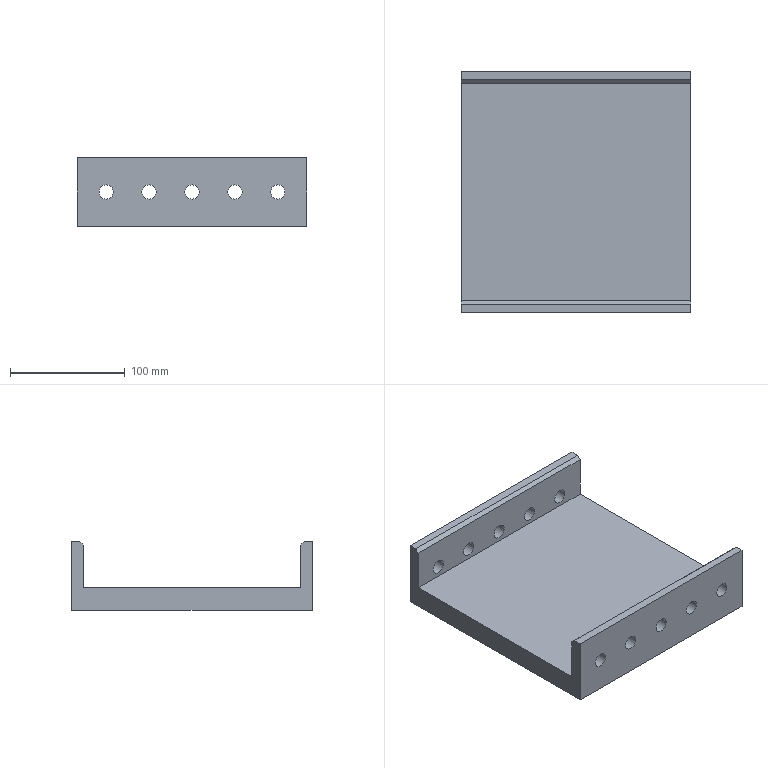Part | NX | features SIMPLE HOLE 15, DATUM_CSYS 7, SKETCH 6, EXTRACT_BODY 5, EXTRACT_DATUM_AXIS 5, EXTRACT_FACE 5, HOLE PACKAGE 5, Instance Feature 4, CHAMFER 2, Delete Body 2, EXTRUDE 2, Container 1, Geometry Instance 1, Pattern Feature 1, SUBTRACT 1 | 1 solid | 22 faces | box 200 x 210 x 60 mm | volume 985928 mm3 | plane 12 | cylinder 10 | commonest cylinder face diameters 12.5 x10
STEP:
#1=CARTESIAN_POINT('',(25.,200.,36.25));
#2=VERTEX_POINT('',#1);
#3=CARTESIAN_POINT('',(25.,200.,30.));
#4=DIRECTION('',(0.,1.,0.));
#5=DIRECTION('',(0.,0.,1.));
#6=AXIS2_PLACEMENT_3D('',#3,#4,#5);
#7=CIRCLE('',#6,6.25);
#8=EDGE_CURVE('',#2,#2,#7,.T.);
#9=ORIENTED_EDGE('',*,*,#8,.T.);
#10=EDGE_LOOP('',(#9));
#11=FACE_BOUND('',#10,.T.);
#12=CARTESIAN_POINT('',(62.5,200.,36.25));
#13=VERTEX_POINT('',#12);
#14=CARTESIAN_POINT('',(62.5,200.,30.));
#15=DIRECTION('',(0.,1.,0.));
#16=DIRECTION('',(0.,0.,1.));
#17=AXIS2_PLACEMENT_3D('',#14,#15,#16);
#18=CIRCLE('',#17,6.25);
#19=EDGE_CURVE('',#13,#13,#18,.T.);
#20=ORIENTED_EDGE('',*,*,#19,.T.);
#21=EDGE_LOOP('',(#20));
#22=FACE_BOUND('',#21,.T.);
#23=CARTESIAN_POINT('',(100.,200.,36.25));
#24=VERTEX_POINT('',#23);
#25=CARTESIAN_POINT('',(100.,200.,30.));
#26=DIRECTION('',(0.,1.,0.));
#27=DIRECTION('',(0.,0.,1.));
#28=AXIS2_PLACEMENT_3D('',#25,#26,#27);
#29=CIRCLE('',#28,6.25);
#30=EDGE_CURVE('',#24,#24,#29,.T.);
#31=ORIENTED_EDGE('',*,*,#30,.T.);
#32=EDGE_LOOP('',(#31));
#33=FACE_BOUND('',#32,.T.);
#34=CARTESIAN_POINT('',(137.5,200.,36.25));
#35=VERTEX_POINT('',#34);
#36=CARTESIAN_POINT('',(137.5,200.,30.));
#37=DIRECTION('',(0.,1.,0.));
#38=DIRECTION('',(0.,0.,1.));
#39=AXIS2_PLACEMENT_3D('',#36,#37,#38);
#40=CIRCLE('',#39,6.25);
#41=EDGE_CURVE('',#35,#35,#40,.T.);
#42=ORIENTED_EDGE('',*,*,#41,.T.);
#43=EDGE_LOOP('',(#42));
#44=FACE_BOUND('',#43,.T.);
#45=CARTESIAN_POINT('',(175.,200.,36.25));
#46=VERTEX_POINT('',#45);
#47=CARTESIAN_POINT('',(175.,200.,30.));
#48=DIRECTION('',(0.,1.,0.));
#49=DIRECTION('',(0.,0.,1.));
#50=AXIS2_PLACEMENT_3D('',#47,#48,#49);
#51=CIRCLE('',#50,6.25);
#52=EDGE_CURVE('',#46,#46,#51,.T.);
#53=ORIENTED_EDGE('',*,*,#52,.T.);
#54=EDGE_LOOP('',(#53));
#55=FACE_BOUND('',#54,.T.);
#56=CARTESIAN_POINT('',(200.,200.,57.));
#57=VERTEX_POINT('',#56);
#58=CARTESIAN_POINT('',(200.,200.,20.));
#59=VERTEX_POINT('',#58);
#60=CARTESIAN_POINT('',(200.,200.,60.));
#61=DIRECTION('',(0.,0.,-1.));
#62=VECTOR('',#61,1000.);
#63=LINE('',#60,#62);
#64=EDGE_CURVE('',#57,#59,#63,.T.);
#65=ORIENTED_EDGE('',*,*,#64,.F.);
#66=CARTESIAN_POINT('',(0.,200.,57.));
#67=VERTEX_POINT('',#66);
#68=CARTESIAN_POINT('',(200.,200.,57.));
#69=DIRECTION('',(-1.,0.,0.));
#70=VECTOR('',#69,1000.);
#71=LINE('',#68,#70);
#72=EDGE_CURVE('',#57,#67,#71,.T.);
#73=ORIENTED_EDGE('',*,*,#72,.T.);
#74=CARTESIAN_POINT('',(0.,200.,20.));
#75=VERTEX_POINT('',#74);
#76=CARTESIAN_POINT('',(0.,200.,60.));
#77=DIRECTION('',(0.,0.,-1.));
#78=VECTOR('',#77,1000.);
#79=LINE('',#76,#78);
#80=EDGE_CURVE('',#67,#75,#79,.T.);
#81=ORIENTED_EDGE('',*,*,#80,.T.);
#82=CARTESIAN_POINT('',(200.,200.,20.));
#83=DIRECTION('',(-1.,0.,0.));
#84=VECTOR('',#83,1000.);
#85=LINE('',#82,#84);
#86=EDGE_CURVE('',#59,#75,#85,.T.);
#87=ORIENTED_EDGE('',*,*,#86,.F.);
#88=EDGE_LOOP('',(#65,#73,#81,#87));
#89=FACE_BOUND('',#88,.T.);
#90=CARTESIAN_POINT('',(200.,200.,60.));
#91=DIRECTION('',(0.,1.,0.));
#92=DIRECTION('',(0.,0.,1.));
#93=AXIS2_PLACEMENT_3D('',#90,#91,#92);
#94=PLANE('',#93);
#95=ADVANCED_FACE('',(#11,#22,#33,#44,#55,#89),#94,.F.);
#96=CARTESIAN_POINT('',(25.,10.,36.25));
#97=VERTEX_POINT('',#96);
#98=CARTESIAN_POINT('',(25.,10.,30.));
#99=DIRECTION('',(0.,1.,0.));
#100=DIRECTION('',(0.,0.,1.));
#101=AXIS2_PLACEMENT_3D('',#98,#99,#100);
#102=CIRCLE('',#101,6.25);
#103=EDGE_CURVE('',#97,#97,#102,.F.);
#104=ORIENTED_EDGE('',*,*,#103,.T.);
#105=EDGE_LOOP('',(#104));
#106=FACE_BOUND('',#105,.T.);
#107=CARTESIAN_POINT('',(62.5,10.,36.25));
#108=VERTEX_POINT('',#107);
#109=CARTESIAN_POINT('',(62.5,10.,30.));
#110=DIRECTION('',(0.,1.,0.));
#111=DIRECTION('',(0.,0.,1.));
#112=AXIS2_PLACEMENT_3D('',#109,#110,#111);
#113=CIRCLE('',#112,6.25);
#114=EDGE_CURVE('',#108,#108,#113,.F.);
#115=ORIENTED_EDGE('',*,*,#114,.T.);
#116=EDGE_LOOP('',(#115));
#117=FACE_BOUND('',#116,.T.);
#118=CARTESIAN_POINT('',(100.,10.,36.25));
#119=VERTEX_POINT('',#118);
#120=CARTESIAN_POINT('',(100.,10.,30.));
#121=DIRECTION('',(0.,1.,0.));
#122=DIRECTION('',(0.,0.,1.));
#123=AXIS2_PLACEMENT_3D('',#120,#121,#122);
#124=CIRCLE('',#123,6.25);
#125=EDGE_CURVE('',#119,#119,#124,.F.);
#126=ORIENTED_EDGE('',*,*,#125,.T.);
#127=EDGE_LOOP('',(#126));
#128=FACE_BOUND('',#127,.T.);
#129=CARTESIAN_POINT('',(175.,10.,36.25));
#130=VERTEX_POINT('',#129);
#131=CARTESIAN_POINT('',(175.,10.,30.));
#132=DIRECTION('',(0.,1.,0.));
#133=DIRECTION('',(0.,0.,1.));
#134=AXIS2_PLACEMENT_3D('',#131,#132,#133);
#135=CIRCLE('',#134,6.25);
#136=EDGE_CURVE('',#130,#130,#135,.F.);
#137=ORIENTED_EDGE('',*,*,#136,.T.);
#138=EDGE_LOOP('',(#137));
#139=FACE_BOUND('',#138,.T.);
#140=CARTESIAN_POINT('',(137.5,10.,36.25));
#141=VERTEX_POINT('',#140);
#142=CARTESIAN_POINT('',(137.5,10.,30.));
#143=DIRECTION('',(0.,1.,0.));
#144=DIRECTION('',(0.,0.,1.));
#145=AXIS2_PLACEMENT_3D('',#142,#143,#144);
#146=CIRCLE('',#145,6.25);
#147=EDGE_CURVE('',#141,#141,#146,.F.);
#148=ORIENTED_EDGE('',*,*,#147,.T.);
#149=EDGE_LOOP('',(#148));
#150=FACE_BOUND('',#149,.T.);
#151=CARTESIAN_POINT('',(0.,10.,20.));
#152=VERTEX_POINT('',#151);
#153=CARTESIAN_POINT('',(0.,10.,57.));
#154=VERTEX_POINT('',#153);
#155=CARTESIAN_POINT('',(0.,10.,10.));
#156=DIRECTION('',(0.,0.,1.));
#157=VECTOR('',#156,1000.);
#158=LINE('',#155,#157);
#159=EDGE_CURVE('',#152,#154,#158,.T.);
#160=ORIENTED_EDGE('',*,*,#159,.T.);
#161=CARTESIAN_POINT('',(200.,10.,57.));
#162=VERTEX_POINT('',#161);
#163=CARTESIAN_POINT('',(200.,10.,57.));
#164=DIRECTION('',(1.,0.,0.));
#165=VECTOR('',#164,1000.);
#166=LINE('',#163,#165);
#167=EDGE_CURVE('',#154,#162,#166,.T.);
#168=ORIENTED_EDGE('',*,*,#167,.T.);
#169=CARTESIAN_POINT('',(200.,10.,20.));
#170=VERTEX_POINT('',#169);
#171=CARTESIAN_POINT('',(200.,10.,10.));
#172=DIRECTION('',(0.,0.,1.));
#173=VECTOR('',#172,1000.);
#174=LINE('',#171,#173);
#175=EDGE_CURVE('',#170,#162,#174,.T.);
#176=ORIENTED_EDGE('',*,*,#175,.F.);
#177=CARTESIAN_POINT('',(0.,10.,20.));
#178=DIRECTION('',(1.,0.,0.));
#179=VECTOR('',#178,1000.);
#180=LINE('',#177,#179);
#181=EDGE_CURVE('',#152,#170,#180,.T.);
#182=ORIENTED_EDGE('',*,*,#181,.F.);
#183=EDGE_LOOP('',(#160,#168,#176,#182));
#184=FACE_BOUND('',#183,.T.);
#185=CARTESIAN_POINT('',(200.,10.,10.));
#186=DIRECTION('',(0.,-1.,0.));
#187=DIRECTION('',(0.,0.,-1.));
#188=AXIS2_PLACEMENT_3D('',#185,#186,#187);
#189=PLANE('',#188);
#190=ADVANCED_FACE('',(#106,#117,#128,#139,#150,#184),#189,.F.);
#191=CARTESIAN_POINT('',(137.5,0.,23.75));
#192=VERTEX_POINT('',#191);
#193=CARTESIAN_POINT('',(137.5,0.,30.));
#194=DIRECTION('',(0.,-1.,0.));
#195=DIRECTION('',(0.,0.,-1.));
#196=AXIS2_PLACEMENT_3D('',#193,#194,#195);
#197=CIRCLE('',#196,6.25);
#198=EDGE_CURVE('',#192,#192,#197,.T.);
#199=ORIENTED_EDGE('',*,*,#198,.F.);
#200=EDGE_LOOP('',(#199));
#201=FACE_BOUND('',#200,.T.);
#202=CARTESIAN_POINT('',(175.,0.,23.75));
#203=VERTEX_POINT('',#202);
#204=CARTESIAN_POINT('',(175.,0.,30.));
#205=DIRECTION('',(0.,-1.,0.));
#206=DIRECTION('',(0.,0.,-1.));
#207=AXIS2_PLACEMENT_3D('',#204,#205,#206);
#208=CIRCLE('',#207,6.25);
#209=EDGE_CURVE('',#203,#203,#208,.T.);
#210=ORIENTED_EDGE('',*,*,#209,.F.);
#211=EDGE_LOOP('',(#210));
#212=FACE_BOUND('',#211,.T.);
#213=CARTESIAN_POINT('',(100.,0.,23.75));
#214=VERTEX_POINT('',#213);
#215=CARTESIAN_POINT('',(100.,0.,30.));
#216=DIRECTION('',(0.,-1.,0.));
#217=DIRECTION('',(0.,0.,-1.));
#218=AXIS2_PLACEMENT_3D('',#215,#216,#217);
#219=CIRCLE('',#218,6.25);
#220=EDGE_CURVE('',#214,#214,#219,.T.);
#221=ORIENTED_EDGE('',*,*,#220,.F.);
#222=EDGE_LOOP('',(#221));
#223=FACE_BOUND('',#222,.T.);
#224=CARTESIAN_POINT('',(62.5,0.,23.75));
#225=VERTEX_POINT('',#224);
#226=CARTESIAN_POINT('',(62.5,0.,30.));
#227=DIRECTION('',(0.,-1.,0.));
#228=DIRECTION('',(0.,0.,-1.));
#229=AXIS2_PLACEMENT_3D('',#226,#227,#228);
#230=CIRCLE('',#229,6.25);
#231=EDGE_CURVE('',#225,#225,#230,.T.);
#232=ORIENTED_EDGE('',*,*,#231,.F.);
#233=EDGE_LOOP('',(#232));
#234=FACE_BOUND('',#233,.T.);
#235=CARTESIAN_POINT('',(25.,0.,23.75));
#236=VERTEX_POINT('',#235);
#237=CARTESIAN_POINT('',(25.,0.,30.));
#238=DIRECTION('',(0.,-1.,0.));
#239=DIRECTION('',(0.,0.,-1.));
#240=AXIS2_PLACEMENT_3D('',#237,#238,#239);
#241=CIRCLE('',#240,6.25);
#242=EDGE_CURVE('',#236,#236,#241,.T.);
#243=ORIENTED_EDGE('',*,*,#242,.F.);
#244=EDGE_LOOP('',(#243));
#245=FACE_BOUND('',#244,.T.);
#246=CARTESIAN_POINT('',(0.,0.,60.));
#247=VERTEX_POINT('',#246);
#248=CARTESIAN_POINT('',(0.,0.,0.));
#249=VERTEX_POINT('',#248);
#250=CARTESIAN_POINT('',(0.,0.,60.));
#251=DIRECTION('',(0.,0.,-1.));
#252=VECTOR('',#251,1000.);
#253=LINE('',#250,#252);
#254=EDGE_CURVE('',#247,#249,#253,.T.);
#255=ORIENTED_EDGE('',*,*,#254,.T.);
#256=CARTESIAN_POINT('',(200.,0.,0.));
#257=VERTEX_POINT('',#256);
#258=CARTESIAN_POINT('',(200.,0.,0.));
#259=DIRECTION('',(-1.,0.,0.));
#260=VECTOR('',#259,1000.);
#261=LINE('',#258,#260);
#262=EDGE_CURVE('',#257,#249,#261,.T.);
#263=ORIENTED_EDGE('',*,*,#262,.F.);
#264=CARTESIAN_POINT('',(200.,0.,60.));
#265=VERTEX_POINT('',#264);
#266=CARTESIAN_POINT('',(200.,0.,60.));
#267=DIRECTION('',(0.,0.,-1.));
#268=VECTOR('',#267,1000.);
#269=LINE('',#266,#268);
#270=EDGE_CURVE('',#265,#257,#269,.T.);
#271=ORIENTED_EDGE('',*,*,#270,.F.);
#272=CARTESIAN_POINT('',(200.,0.,60.));
#273=DIRECTION('',(-1.,0.,0.));
#274=VECTOR('',#273,1000.);
#275=LINE('',#272,#274);
#276=EDGE_CURVE('',#265,#247,#275,.T.);
#277=ORIENTED_EDGE('',*,*,#276,.T.);
#278=EDGE_LOOP('',(#255,#263,#271,#277));
#279=FACE_BOUND('',#278,.T.);
#280=CARTESIAN_POINT('',(200.,0.,60.));
#281=DIRECTION('',(0.,1.,0.));
#282=DIRECTION('',(0.,0.,1.));
#283=AXIS2_PLACEMENT_3D('',#280,#281,#282);
#284=PLANE('',#283);
#285=ADVANCED_FACE('',(#201,#212,#223,#234,#245,#279),#284,.F.);
#286=CARTESIAN_POINT('',(0.,210.,0.));
#287=VERTEX_POINT('',#286);
#288=CARTESIAN_POINT('',(0.,0.,0.));
#289=DIRECTION('',(0.,1.,0.));
#290=VECTOR('',#289,1000.);
#291=LINE('',#288,#290);
#292=EDGE_CURVE('',#249,#287,#291,.T.);
#293=ORIENTED_EDGE('',*,*,#292,.T.);
#294=CARTESIAN_POINT('',(200.,210.,0.));
#295=VERTEX_POINT('',#294);
#296=CARTESIAN_POINT('',(200.,210.,0.));
#297=DIRECTION('',(-1.,0.,0.));
#298=VECTOR('',#297,1000.);
#299=LINE('',#296,#298);
#300=EDGE_CURVE('',#295,#287,#299,.T.);
#301=ORIENTED_EDGE('',*,*,#300,.F.);
#302=CARTESIAN_POINT('',(200.,0.,0.));
#303=DIRECTION('',(0.,1.,0.));
#304=VECTOR('',#303,1000.);
#305=LINE('',#302,#304);
#306=EDGE_CURVE('',#257,#295,#305,.T.);
#307=ORIENTED_EDGE('',*,*,#306,.F.);
#308=ORIENTED_EDGE('',*,*,#262,.T.);
#309=EDGE_LOOP('',(#293,#301,#307,#308));
#310=FACE_BOUND('',#309,.T.);
#311=CARTESIAN_POINT('',(200.,0.,0.));
#312=DIRECTION('',(0.,0.,1.));
#313=DIRECTION('',(0.,-1.,0.));
#314=AXIS2_PLACEMENT_3D('',#311,#312,#313);
#315=PLANE('',#314);
#316=ADVANCED_FACE('',(#310),#315,.F.);
#317=CARTESIAN_POINT('',(175.,210.,23.75));
#318=VERTEX_POINT('',#317);
#319=CARTESIAN_POINT('',(175.,210.,30.));
#320=DIRECTION('',(0.,-1.,0.));
#321=DIRECTION('',(0.,0.,-1.));
#322=AXIS2_PLACEMENT_3D('',#319,#320,#321);
#323=CIRCLE('',#322,6.25);
#324=EDGE_CURVE('',#318,#318,#323,.F.);
#325=ORIENTED_EDGE('',*,*,#324,.F.);
#326=EDGE_LOOP('',(#325));
#327=FACE_BOUND('',#326,.T.);
#328=CARTESIAN_POINT('',(137.5,210.,23.75));
#329=VERTEX_POINT('',#328);
#330=CARTESIAN_POINT('',(137.5,210.,30.));
#331=DIRECTION('',(0.,-1.,0.));
#332=DIRECTION('',(0.,0.,-1.));
#333=AXIS2_PLACEMENT_3D('',#330,#331,#332);
#334=CIRCLE('',#333,6.25);
#335=EDGE_CURVE('',#329,#329,#334,.F.);
#336=ORIENTED_EDGE('',*,*,#335,.F.);
#337=EDGE_LOOP('',(#336));
#338=FACE_BOUND('',#337,.T.);
#339=CARTESIAN_POINT('',(100.,210.,23.75));
#340=VERTEX_POINT('',#339);
#341=CARTESIAN_POINT('',(100.,210.,30.));
#342=DIRECTION('',(0.,-1.,0.));
#343=DIRECTION('',(0.,0.,-1.));
#344=AXIS2_PLACEMENT_3D('',#341,#342,#343);
#345=CIRCLE('',#344,6.25);
#346=EDGE_CURVE('',#340,#340,#345,.F.);
#347=ORIENTED_EDGE('',*,*,#346,.F.);
#348=EDGE_LOOP('',(#347));
#349=FACE_BOUND('',#348,.T.);
#350=CARTESIAN_POINT('',(62.5,210.,23.75));
#351=VERTEX_POINT('',#350);
#352=CARTESIAN_POINT('',(62.5,210.,30.));
#353=DIRECTION('',(0.,-1.,0.));
#354=DIRECTION('',(0.,0.,-1.));
#355=AXIS2_PLACEMENT_3D('',#352,#353,#354);
#356=CIRCLE('',#355,6.25);
#357=EDGE_CURVE('',#351,#351,#356,.F.);
#358=ORIENTED_EDGE('',*,*,#357,.F.);
#359=EDGE_LOOP('',(#358));
#360=FACE_BOUND('',#359,.T.);
#361=CARTESIAN_POINT('',(25.,210.,23.75));
#362=VERTEX_POINT('',#361);
#363=CARTESIAN_POINT('',(25.,210.,30.));
#364=DIRECTION('',(0.,-1.,0.));
#365=DIRECTION('',(0.,0.,-1.));
#366=AXIS2_PLACEMENT_3D('',#363,#364,#365);
#367=CIRCLE('',#366,6.25);
#368=EDGE_CURVE('',#362,#362,#367,.T.);
#369=ORIENTED_EDGE('',*,*,#368,.T.);
#370=EDGE_LOOP('',(#369));
#371=FACE_BOUND('',#370,.T.);
#372=CARTESIAN_POINT('',(0.,210.,60.));
#373=VERTEX_POINT('',#372);
#374=CARTESIAN_POINT('',(0.,210.,0.));
#375=DIRECTION('',(0.,0.,1.));
#376=VECTOR('',#375,1000.);
#377=LINE('',#374,#376);
#378=EDGE_CURVE('',#287,#373,#377,.T.);
#379=ORIENTED_EDGE('',*,*,#378,.T.);
#380=CARTESIAN_POINT('',(200.,210.,60.));
#381=VERTEX_POINT('',#380);
#382=CARTESIAN_POINT('',(200.,210.,60.));
#383=DIRECTION('',(-1.,0.,0.));
#384=VECTOR('',#383,1000.);
#385=LINE('',#382,#384);
#386=EDGE_CURVE('',#381,#373,#385,.T.);
#387=ORIENTED_EDGE('',*,*,#386,.F.);
#388=CARTESIAN_POINT('',(200.,210.,0.));
#389=DIRECTION('',(0.,0.,1.));
#390=VECTOR('',#389,1000.);
#391=LINE('',#388,#390);
#392=EDGE_CURVE('',#295,#381,#391,.T.);
#393=ORIENTED_EDGE('',*,*,#392,.F.);
#394=ORIENTED_EDGE('',*,*,#300,.T.);
#395=EDGE_LOOP('',(#379,#387,#393,#394));
#396=FACE_BOUND('',#395,.T.);
#397=CARTESIAN_POINT('',(200.,210.,0.));
#398=DIRECTION('',(0.,-1.,0.));
#399=DIRECTION('',(0.,0.,-1.));
#400=AXIS2_PLACEMENT_3D('',#397,#398,#399);
#401=PLANE('',#400);
#402=ADVANCED_FACE('',(#327,#338,#349,#360,#371,#396),#401,.F.);
#403=CARTESIAN_POINT('',(0.,203.,60.));
#404=VERTEX_POINT('',#403);
#405=CARTESIAN_POINT('',(0.,210.,60.));
#406=DIRECTION('',(0.,-1.,0.));
#407=VECTOR('',#406,1000.);
#408=LINE('',#405,#407);
#409=EDGE_CURVE('',#373,#404,#408,.T.);
#410=ORIENTED_EDGE('',*,*,#409,.T.);
#411=CARTESIAN_POINT('',(200.,203.,60.));
#412=VERTEX_POINT('',#411);
#413=CARTESIAN_POINT('',(200.,203.,60.));
#414=DIRECTION('',(1.,0.,0.));
#415=VECTOR('',#414,1000.);
#416=LINE('',#413,#415);
#417=EDGE_CURVE('',#404,#412,#416,.T.);
#418=ORIENTED_EDGE('',*,*,#417,.T.);
#419=CARTESIAN_POINT('',(200.,210.,60.));
#420=DIRECTION('',(0.,-1.,0.));
#421=VECTOR('',#420,1000.);
#422=LINE('',#419,#421);
#423=EDGE_CURVE('',#381,#412,#422,.T.);
#424=ORIENTED_EDGE('',*,*,#423,.F.);
#425=ORIENTED_EDGE('',*,*,#386,.T.);
#426=EDGE_LOOP('',(#410,#418,#424,#425));
#427=FACE_BOUND('',#426,.T.);
#428=CARTESIAN_POINT('',(200.,210.,60.));
#429=DIRECTION('',(0.,0.,-1.));
#430=DIRECTION('',(-1.,0.,0.));
#431=AXIS2_PLACEMENT_3D('',#428,#429,#430);
#432=PLANE('',#431);
#433=ADVANCED_FACE('',(#427),#432,.F.);
#434=CARTESIAN_POINT('',(200.,7.,60.));
#435=VERTEX_POINT('',#434);
#436=CARTESIAN_POINT('',(200.,10.,60.));
#437=DIRECTION('',(0.,-1.,0.));
#438=VECTOR('',#437,1000.);
#439=LINE('',#436,#438);
#440=EDGE_CURVE('',#435,#265,#439,.T.);
#441=ORIENTED_EDGE('',*,*,#440,.F.);
#442=CARTESIAN_POINT('',(0.,7.,60.));
#443=VERTEX_POINT('',#442);
#444=CARTESIAN_POINT('',(200.,7.,60.));
#445=DIRECTION('',(-1.,0.,0.));
#446=VECTOR('',#445,1000.);
#447=LINE('',#444,#446);
#448=EDGE_CURVE('',#435,#443,#447,.T.);
#449=ORIENTED_EDGE('',*,*,#448,.T.);
#450=CARTESIAN_POINT('',(0.,10.,60.));
#451=DIRECTION('',(0.,-1.,0.));
#452=VECTOR('',#451,1000.);
#453=LINE('',#450,#452);
#454=EDGE_CURVE('',#443,#247,#453,.T.);
#455=ORIENTED_EDGE('',*,*,#454,.T.);
#456=ORIENTED_EDGE('',*,*,#276,.F.);
#457=EDGE_LOOP('',(#441,#449,#455,#456));
#458=FACE_BOUND('',#457,.T.);
#459=CARTESIAN_POINT('',(200.,10.,60.));
#460=DIRECTION('',(0.,0.,-1.));
#461=DIRECTION('',(-1.,0.,0.));
#462=AXIS2_PLACEMENT_3D('',#459,#460,#461);
#463=PLANE('',#462);
#464=ADVANCED_FACE('',(#458),#463,.F.);
#465=ORIENTED_EDGE('',*,*,#175,.T.);
#466=CARTESIAN_POINT('',(200.,33.5,33.5));
#467=DIRECTION('',(0.,0.7071,-0.7071));
#468=VECTOR('',#467,1000.);
#469=LINE('',#466,#468);
#470=EDGE_CURVE('',#162,#435,#469,.F.);
#471=ORIENTED_EDGE('',*,*,#470,.T.);
#472=ORIENTED_EDGE('',*,*,#440,.T.);
#473=ORIENTED_EDGE('',*,*,#270,.T.);
#474=ORIENTED_EDGE('',*,*,#306,.T.);
#475=ORIENTED_EDGE('',*,*,#392,.T.);
#476=ORIENTED_EDGE('',*,*,#423,.T.);
#477=CARTESIAN_POINT('',(200.,71.5,-71.5));
#478=DIRECTION('',(0.,0.7071,0.7071));
#479=VECTOR('',#478,1000.);
#480=LINE('',#477,#479);
#481=EDGE_CURVE('',#412,#57,#480,.F.);
#482=ORIENTED_EDGE('',*,*,#481,.T.);
#483=ORIENTED_EDGE('',*,*,#64,.T.);
#484=CARTESIAN_POINT('',(200.,10.,20.));
#485=DIRECTION('',(0.,1.,0.));
#486=VECTOR('',#485,1000.);
#487=LINE('',#484,#486);
#488=EDGE_CURVE('',#170,#59,#487,.T.);
#489=ORIENTED_EDGE('',*,*,#488,.F.);
#490=EDGE_LOOP('',(#465,#471,#472,#473,#474,#475,#476,#482,#483,#489));
#491=FACE_BOUND('',#490,.T.);
#492=CARTESIAN_POINT('',(200.,0.,0.));
#493=DIRECTION('',(1.,0.,0.));
#494=DIRECTION('',(0.,0.,-1.));
#495=AXIS2_PLACEMENT_3D('',#492,#493,#494);
#496=PLANE('',#495);
#497=ADVANCED_FACE('',(#491),#496,.T.);
#498=ORIENTED_EDGE('',*,*,#454,.F.);
#499=CARTESIAN_POINT('',(0.,7.,60.));
#500=DIRECTION('',(0.,-0.7071,0.7071));
#501=VECTOR('',#500,1000.);
#502=LINE('',#499,#501);
#503=EDGE_CURVE('',#443,#154,#502,.F.);
#504=ORIENTED_EDGE('',*,*,#503,.T.);
#505=ORIENTED_EDGE('',*,*,#159,.F.);
#506=CARTESIAN_POINT('',(0.,200.,20.));
#507=DIRECTION('',(0.,-1.,0.));
#508=VECTOR('',#507,1000.);
#509=LINE('',#506,#508);
#510=EDGE_CURVE('',#75,#152,#509,.T.);
#511=ORIENTED_EDGE('',*,*,#510,.F.);
#512=ORIENTED_EDGE('',*,*,#80,.F.);
#513=CARTESIAN_POINT('',(0.,200.,57.));
#514=DIRECTION('',(0.,-0.7071,-0.7071));
#515=VECTOR('',#514,1000.);
#516=LINE('',#513,#515);
#517=EDGE_CURVE('',#67,#404,#516,.F.);
#518=ORIENTED_EDGE('',*,*,#517,.T.);
#519=ORIENTED_EDGE('',*,*,#409,.F.);
#520=ORIENTED_EDGE('',*,*,#378,.F.);
#521=ORIENTED_EDGE('',*,*,#292,.F.);
#522=ORIENTED_EDGE('',*,*,#254,.F.);
#523=EDGE_LOOP('',(#498,#504,#505,#511,#512,#518,#519,#520,#521,#522));
#524=FACE_BOUND('',#523,.T.);
#525=CARTESIAN_POINT('',(0.,0.,0.));
#526=DIRECTION('',(1.,0.,0.));
#527=DIRECTION('',(0.,0.,-1.));
#528=AXIS2_PLACEMENT_3D('',#525,#526,#527);
#529=PLANE('',#528);
#530=ADVANCED_FACE('',(#524),#529,.F.);
#531=ORIENTED_EDGE('',*,*,#368,.F.);
#532=EDGE_LOOP('',(#531));
#533=FACE_BOUND('',#532,.T.);
#534=ORIENTED_EDGE('',*,*,#8,.F.);
#535=EDGE_LOOP('',(#534));
#536=FACE_BOUND('',#535,.T.);
#537=CARTESIAN_POINT('',(25.,200.,30.));
#538=DIRECTION('',(0.,1.,0.));
#539=DIRECTION('',(0.,0.,1.));
#540=AXIS2_PLACEMENT_3D('',#537,#538,#539);
#541=CYLINDRICAL_SURFACE('',#540,6.25);
#542=ADVANCED_FACE('',(#533,#536),#541,.F.);
#543=ORIENTED_EDGE('',*,*,#242,.T.);
#544=EDGE_LOOP('',(#543));
#545=FACE_BOUND('',#544,.T.);
#546=ORIENTED_EDGE('',*,*,#103,.F.);
#547=EDGE_LOOP('',(#546));
#548=FACE_BOUND('',#547,.T.);
#549=CARTESIAN_POINT('',(25.,10.,30.));
#550=DIRECTION('',(0.,-1.,0.));
#551=DIRECTION('',(0.,0.,1.));
#552=AXIS2_PLACEMENT_3D('',#549,#550,#551);
#553=CYLINDRICAL_SURFACE('',#552,6.25);
#554=ADVANCED_FACE('',(#545,#548),#553,.F.);
#555=ORIENTED_EDGE('',*,*,#357,.T.);
#556=EDGE_LOOP('',(#555));
#557=FACE_BOUND('',#556,.T.);
#558=ORIENTED_EDGE('',*,*,#19,.F.);
#559=EDGE_LOOP('',(#558));
#560=FACE_BOUND('',#559,.T.);
#561=CARTESIAN_POINT('',(62.5,200.,30.));
#562=DIRECTION('',(0.,1.,0.));
#563=DIRECTION('',(0.,0.,1.));
#564=AXIS2_PLACEMENT_3D('',#561,#562,#563);
#565=CYLINDRICAL_SURFACE('',#564,6.25);
#566=ADVANCED_FACE('',(#557,#560),#565,.F.);
#567=ORIENTED_EDGE('',*,*,#346,.T.);
#568=EDGE_LOOP('',(#567));
#569=FACE_BOUND('',#568,.T.);
#570=ORIENTED_EDGE('',*,*,#30,.F.);
#571=EDGE_LOOP('',(#570));
#572=FACE_BOUND('',#571,.T.);
#573=CARTESIAN_POINT('',(100.,200.,30.));
#574=DIRECTION('',(0.,1.,0.));
#575=DIRECTION('',(0.,0.,1.));
#576=AXIS2_PLACEMENT_3D('',#573,#574,#575);
#577=CYLINDRICAL_SURFACE('',#576,6.25);
#578=ADVANCED_FACE('',(#569,#572),#577,.F.);
#579=ORIENTED_EDGE('',*,*,#335,.T.);
#580=EDGE_LOOP('',(#579));
#581=FACE_BOUND('',#580,.T.);
#582=ORIENTED_EDGE('',*,*,#41,.F.);
#583=EDGE_LOOP('',(#582));
#584=FACE_BOUND('',#583,.T.);
#585=CARTESIAN_POINT('',(137.5,200.,30.));
#586=DIRECTION('',(0.,1.,0.));
#587=DIRECTION('',(0.,0.,1.));
#588=AXIS2_PLACEMENT_3D('',#585,#586,#587);
#589=CYLINDRICAL_SURFACE('',#588,6.25);
#590=ADVANCED_FACE('',(#581,#584),#589,.F.);
#591=ORIENTED_EDGE('',*,*,#324,.T.);
#592=EDGE_LOOP('',(#591));
#593=FACE_BOUND('',#592,.T.);
#594=ORIENTED_EDGE('',*,*,#52,.F.);
#595=EDGE_LOOP('',(#594));
#596=FACE_BOUND('',#595,.T.);
#597=CARTESIAN_POINT('',(175.,200.,30.));
#598=DIRECTION('',(0.,1.,0.));
#599=DIRECTION('',(0.,0.,1.));
#600=AXIS2_PLACEMENT_3D('',#597,#598,#599);
#601=CYLINDRICAL_SURFACE('',#600,6.25);
#602=ADVANCED_FACE('',(#593,#596),#601,.F.);
#603=ORIENTED_EDGE('',*,*,#231,.T.);
#604=EDGE_LOOP('',(#603));
#605=FACE_BOUND('',#604,.T.);
#606=ORIENTED_EDGE('',*,*,#114,.F.);
#607=EDGE_LOOP('',(#606));
#608=FACE_BOUND('',#607,.T.);
#609=CARTESIAN_POINT('',(62.5,10.,30.));
#610=DIRECTION('',(0.,-1.,0.));
#611=DIRECTION('',(0.,0.,1.));
#612=AXIS2_PLACEMENT_3D('',#609,#610,#611);
#613=CYLINDRICAL_SURFACE('',#612,6.25);
#614=ADVANCED_FACE('',(#605,#608),#613,.F.);
#615=ORIENTED_EDGE('',*,*,#220,.T.);
#616=EDGE_LOOP('',(#615));
#617=FACE_BOUND('',#616,.T.);
#618=ORIENTED_EDGE('',*,*,#125,.F.);
#619=EDGE_LOOP('',(#618));
#620=FACE_BOUND('',#619,.T.);
#621=CARTESIAN_POINT('',(100.,10.,30.));
#622=DIRECTION('',(0.,-1.,0.));
#623=DIRECTION('',(0.,0.,1.));
#624=AXIS2_PLACEMENT_3D('',#621,#622,#623);
#625=CYLINDRICAL_SURFACE('',#624,6.25);
#626=ADVANCED_FACE('',(#617,#620),#625,.F.);
#627=ORIENTED_EDGE('',*,*,#209,.T.);
#628=EDGE_LOOP('',(#627));
#629=FACE_BOUND('',#628,.T.);
#630=ORIENTED_EDGE('',*,*,#136,.F.);
#631=EDGE_LOOP('',(#630));
#632=FACE_BOUND('',#631,.T.);
#633=CARTESIAN_POINT('',(175.,10.,30.));
#634=DIRECTION('',(0.,-1.,0.));
#635=DIRECTION('',(0.,0.,1.));
#636=AXIS2_PLACEMENT_3D('',#633,#634,#635);
#637=CYLINDRICAL_SURFACE('',#636,6.25);
#638=ADVANCED_FACE('',(#629,#632),#637,.F.);
#639=ORIENTED_EDGE('',*,*,#198,.T.);
#640=EDGE_LOOP('',(#639));
#641=FACE_BOUND('',#640,.T.);
#642=ORIENTED_EDGE('',*,*,#147,.F.);
#643=EDGE_LOOP('',(#642));
#644=FACE_BOUND('',#643,.T.);
#645=CARTESIAN_POINT('',(137.5,10.,30.));
#646=DIRECTION('',(0.,-1.,0.));
#647=DIRECTION('',(0.,0.,1.));
#648=AXIS2_PLACEMENT_3D('',#645,#646,#647);
#649=CYLINDRICAL_SURFACE('',#648,6.25);
#650=ADVANCED_FACE('',(#641,#644),#649,.F.);
#651=ORIENTED_EDGE('',*,*,#510,.T.);
#652=ORIENTED_EDGE('',*,*,#181,.T.);
#653=ORIENTED_EDGE('',*,*,#488,.T.);
#654=ORIENTED_EDGE('',*,*,#86,.T.);
#655=EDGE_LOOP('',(#651,#652,#653,#654));
#656=FACE_BOUND('',#655,.T.);
#657=CARTESIAN_POINT('',(0.,0.,20.));
#658=DIRECTION('',(0.,0.,1.));
#659=DIRECTION('',(1.,0.,0.));
#660=AXIS2_PLACEMENT_3D('',#657,#658,#659);
#661=PLANE('',#660);
#662=ADVANCED_FACE('',(#656),#661,.T.);
#663=ORIENTED_EDGE('',*,*,#481,.F.);
#664=ORIENTED_EDGE('',*,*,#417,.F.);
#665=ORIENTED_EDGE('',*,*,#517,.F.);
#666=ORIENTED_EDGE('',*,*,#72,.F.);
#667=EDGE_LOOP('',(#663,#664,#665,#666));
#668=FACE_BOUND('',#667,.T.);
#669=CARTESIAN_POINT('',(200.,200.,57.));
#670=DIRECTION('',(0.,0.7071,-0.7071));
#671=DIRECTION('',(-1.,0.,0.));
#672=AXIS2_PLACEMENT_3D('',#669,#670,#671);
#673=PLANE('',#672);
#674=ADVANCED_FACE('',(#668),#673,.F.);
#675=ORIENTED_EDGE('',*,*,#470,.F.);
#676=ORIENTED_EDGE('',*,*,#167,.F.);
#677=ORIENTED_EDGE('',*,*,#503,.F.);
#678=ORIENTED_EDGE('',*,*,#448,.F.);
#679=EDGE_LOOP('',(#675,#676,#677,#678));
#680=FACE_BOUND('',#679,.T.);
#681=CARTESIAN_POINT('',(200.,7.,60.));
#682=DIRECTION('',(0.,-0.7071,-0.7071));
#683=DIRECTION('',(-1.,0.,0.));
#684=AXIS2_PLACEMENT_3D('',#681,#682,#683);
#685=PLANE('',#684);
#686=ADVANCED_FACE('',(#680),#685,.F.);
#687=CLOSED_SHELL('',(#95,#190,#285,#316,#402,#433,#464,#497,#530,#542,#554,#566,#578,#590,#602,#614,#626,#638,#650,#662,#674,#686));
#688=MANIFOLD_SOLID_BREP('',#687);
#689=(LENGTH_UNIT()NAMED_UNIT(*)SI_UNIT(.MILLI.,.METRE.));
#690=UNCERTAINTY_MEASURE_WITH_UNIT(LENGTH_MEASURE(0.00001),#689,'','');
#691=(NAMED_UNIT(*)PLANE_ANGLE_UNIT()SI_UNIT($,.RADIAN.));
#692=(NAMED_UNIT(*)SI_UNIT($,.STERADIAN.)SOLID_ANGLE_UNIT());
#693=(GEOMETRIC_REPRESENTATION_CONTEXT(3)GLOBAL_UNCERTAINTY_ASSIGNED_CONTEXT((#690))GLOBAL_UNIT_ASSIGNED_CONTEXT((#689,#691,#692))REPRESENTATION_CONTEXT('',''));
#694=ADVANCED_BREP_SHAPE_REPRESENTATION('',(#688),#693);